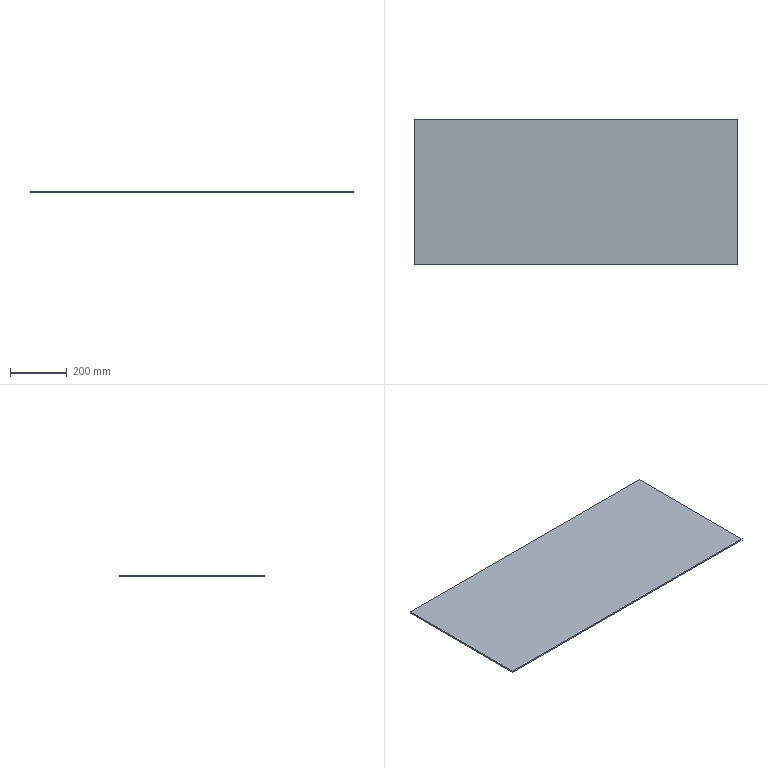Part | SolidWorks | features Extrusion 1, HoleWzd 1 | 1 solid | 6 faces | box 1142 x 513 x 5 mm | volume 2929230 mm3 | plane 6
STEP:
#1=CARTESIAN_POINT('',(571.,-256.5,0.));
#2=VERTEX_POINT('',#1);
#3=CARTESIAN_POINT('',(571.,256.5,0.));
#4=VERTEX_POINT('',#3);
#5=CARTESIAN_POINT('',(571.,256.5,0.));
#6=DIRECTION('',(0.,1.,0.));
#7=VECTOR('',#6,1000.);
#8=LINE('',#5,#7);
#9=EDGE_CURVE('',#2,#4,#8,.T.);
#10=ORIENTED_EDGE('',*,*,#9,.T.);
#11=CARTESIAN_POINT('',(571.,256.5,5.));
#12=VERTEX_POINT('',#11);
#13=CARTESIAN_POINT('',(571.,256.5,5.));
#14=DIRECTION('',(0.,0.,-1.));
#15=VECTOR('',#14,1000.);
#16=LINE('',#13,#15);
#17=EDGE_CURVE('',#12,#4,#16,.T.);
#18=ORIENTED_EDGE('',*,*,#17,.F.);
#19=CARTESIAN_POINT('',(571.,-256.5,5.));
#20=VERTEX_POINT('',#19);
#21=CARTESIAN_POINT('',(571.,256.5,5.));
#22=DIRECTION('',(0.,1.,0.));
#23=VECTOR('',#22,1000.);
#24=LINE('',#21,#23);
#25=EDGE_CURVE('',#20,#12,#24,.T.);
#26=ORIENTED_EDGE('',*,*,#25,.F.);
#27=CARTESIAN_POINT('',(571.,-256.5,5.));
#28=DIRECTION('',(0.,0.,-1.));
#29=VECTOR('',#28,1000.);
#30=LINE('',#27,#29);
#31=EDGE_CURVE('',#20,#2,#30,.T.);
#32=ORIENTED_EDGE('',*,*,#31,.T.);
#33=EDGE_LOOP('',(#10,#18,#26,#32));
#34=FACE_OUTER_BOUND('',#33,.T.);
#35=CARTESIAN_POINT('',(571.,256.5,5.));
#36=DIRECTION('',(-1.,0.,0.));
#37=DIRECTION('',(0.,0.,1.));
#38=AXIS2_PLACEMENT_3D('',#35,#36,#37);
#39=PLANE('',#38);
#40=ADVANCED_FACE('',(#34),#39,.F.);
#41=CARTESIAN_POINT('',(-571.,256.5,0.));
#42=VERTEX_POINT('',#41);
#43=CARTESIAN_POINT('',(-571.,256.5,0.));
#44=DIRECTION('',(-1.,0.,0.));
#45=VECTOR('',#44,1000.);
#46=LINE('',#43,#45);
#47=EDGE_CURVE('',#4,#42,#46,.T.);
#48=ORIENTED_EDGE('',*,*,#47,.T.);
#49=CARTESIAN_POINT('',(-571.,256.5,5.));
#50=VERTEX_POINT('',#49);
#51=CARTESIAN_POINT('',(-571.,256.5,5.));
#52=DIRECTION('',(0.,0.,-1.));
#53=VECTOR('',#52,1000.);
#54=LINE('',#51,#53);
#55=EDGE_CURVE('',#50,#42,#54,.T.);
#56=ORIENTED_EDGE('',*,*,#55,.F.);
#57=CARTESIAN_POINT('',(-571.,256.5,5.));
#58=DIRECTION('',(-1.,0.,0.));
#59=VECTOR('',#58,1000.);
#60=LINE('',#57,#59);
#61=EDGE_CURVE('',#12,#50,#60,.T.);
#62=ORIENTED_EDGE('',*,*,#61,.F.);
#63=ORIENTED_EDGE('',*,*,#17,.T.);
#64=EDGE_LOOP('',(#48,#56,#62,#63));
#65=FACE_OUTER_BOUND('',#64,.T.);
#66=CARTESIAN_POINT('',(-571.,256.5,5.));
#67=DIRECTION('',(0.,-1.,0.));
#68=DIRECTION('',(0.,0.,-1.));
#69=AXIS2_PLACEMENT_3D('',#66,#67,#68);
#70=PLANE('',#69);
#71=ADVANCED_FACE('',(#65),#70,.F.);
#72=CARTESIAN_POINT('',(-571.,-256.5,0.));
#73=VERTEX_POINT('',#72);
#74=CARTESIAN_POINT('',(-571.,256.5,0.));
#75=DIRECTION('',(0.,-1.,0.));
#76=VECTOR('',#75,1000.);
#77=LINE('',#74,#76);
#78=EDGE_CURVE('',#42,#73,#77,.T.);
#79=ORIENTED_EDGE('',*,*,#78,.T.);
#80=CARTESIAN_POINT('',(-571.,-256.5,5.));
#81=VERTEX_POINT('',#80);
#82=CARTESIAN_POINT('',(-571.,-256.5,5.));
#83=DIRECTION('',(0.,0.,-1.));
#84=VECTOR('',#83,1000.);
#85=LINE('',#82,#84);
#86=EDGE_CURVE('',#81,#73,#85,.T.);
#87=ORIENTED_EDGE('',*,*,#86,.F.);
#88=CARTESIAN_POINT('',(-571.,256.5,5.));
#89=DIRECTION('',(0.,-1.,0.));
#90=VECTOR('',#89,1000.);
#91=LINE('',#88,#90);
#92=EDGE_CURVE('',#50,#81,#91,.T.);
#93=ORIENTED_EDGE('',*,*,#92,.F.);
#94=ORIENTED_EDGE('',*,*,#55,.T.);
#95=EDGE_LOOP('',(#79,#87,#93,#94));
#96=FACE_OUTER_BOUND('',#95,.T.);
#97=CARTESIAN_POINT('',(-571.,256.5,5.));
#98=DIRECTION('',(1.,0.,0.));
#99=DIRECTION('',(0.,1.,0.));
#100=AXIS2_PLACEMENT_3D('',#97,#98,#99);
#101=PLANE('',#100);
#102=ADVANCED_FACE('',(#96),#101,.F.);
#103=CARTESIAN_POINT('',(-571.,-256.5,0.));
#104=DIRECTION('',(1.,0.,0.));
#105=VECTOR('',#104,1000.);
#106=LINE('',#103,#105);
#107=EDGE_CURVE('',#73,#2,#106,.T.);
#108=ORIENTED_EDGE('',*,*,#107,.T.);
#109=ORIENTED_EDGE('',*,*,#31,.F.);
#110=CARTESIAN_POINT('',(-571.,-256.5,5.));
#111=DIRECTION('',(1.,0.,0.));
#112=VECTOR('',#111,1000.);
#113=LINE('',#110,#112);
#114=EDGE_CURVE('',#81,#20,#113,.T.);
#115=ORIENTED_EDGE('',*,*,#114,.F.);
#116=ORIENTED_EDGE('',*,*,#86,.T.);
#117=EDGE_LOOP('',(#108,#109,#115,#116));
#118=FACE_OUTER_BOUND('',#117,.T.);
#119=CARTESIAN_POINT('',(-571.,-256.5,5.));
#120=DIRECTION('',(0.,1.,0.));
#121=DIRECTION('',(0.,0.,1.));
#122=AXIS2_PLACEMENT_3D('',#119,#120,#121);
#123=PLANE('',#122);
#124=ADVANCED_FACE('',(#118),#123,.F.);
#125=ORIENTED_EDGE('',*,*,#25,.T.);
#126=ORIENTED_EDGE('',*,*,#61,.T.);
#127=ORIENTED_EDGE('',*,*,#92,.T.);
#128=ORIENTED_EDGE('',*,*,#114,.T.);
#129=EDGE_LOOP('',(#125,#126,#127,#128));
#130=FACE_OUTER_BOUND('',#129,.T.);
#131=CARTESIAN_POINT('',(0.,0.,5.));
#132=DIRECTION('',(0.,0.,1.));
#133=DIRECTION('',(1.,0.,0.));
#134=AXIS2_PLACEMENT_3D('',#131,#132,#133);
#135=PLANE('',#134);
#136=ADVANCED_FACE('',(#130),#135,.T.);
#137=ORIENTED_EDGE('',*,*,#9,.F.);
#138=ORIENTED_EDGE('',*,*,#107,.F.);
#139=ORIENTED_EDGE('',*,*,#78,.F.);
#140=ORIENTED_EDGE('',*,*,#47,.F.);
#141=EDGE_LOOP('',(#137,#138,#139,#140));
#142=FACE_OUTER_BOUND('',#141,.T.);
#143=CARTESIAN_POINT('',(0.,0.,0.));
#144=DIRECTION('',(0.,0.,1.));
#145=DIRECTION('',(1.,0.,0.));
#146=AXIS2_PLACEMENT_3D('',#143,#144,#145);
#147=PLANE('',#146);
#148=ADVANCED_FACE('',(#142),#147,.F.);
#149=CLOSED_SHELL('',(#40,#71,#102,#124,#136,#148));
#150=MANIFOLD_SOLID_BREP('',#149);
#151=CARTESIAN_POINT('',(0.,0.,0.));
#152=DIRECTION('',(0.,0.,1.));
#153=DIRECTION('',(1.,0.,0.));
#154=AXIS2_PLACEMENT_3D('',#151,#152,#153);
#155=(LENGTH_UNIT()NAMED_UNIT(*)SI_UNIT(.MILLI.,.METRE.));
#156=UNCERTAINTY_MEASURE_WITH_UNIT(LENGTH_MEASURE(0.00001),#155,'','');
#157=(NAMED_UNIT(*)PLANE_ANGLE_UNIT()SI_UNIT($,.RADIAN.));
#158=(NAMED_UNIT(*)SI_UNIT($,.STERADIAN.)SOLID_ANGLE_UNIT());
#159=(GEOMETRIC_REPRESENTATION_CONTEXT(3)GLOBAL_UNCERTAINTY_ASSIGNED_CONTEXT((#156))GLOBAL_UNIT_ASSIGNED_CONTEXT((#155,#157,#158))REPRESENTATION_CONTEXT('',''));
#160=ADVANCED_BREP_SHAPE_REPRESENTATION('',(#150,#154),#159);